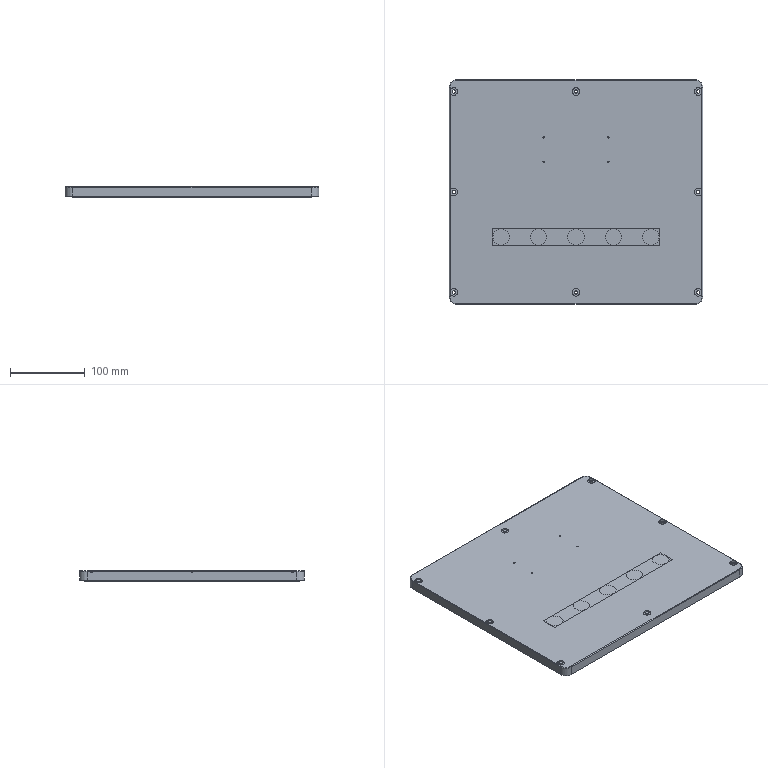Part | 2 solids | 125 faces | box 338 x 300 x 14.5 mm | volume 656011 mm3 | cylinder 57 | plane 52 | cone 12 | torus 4 | commonest cylinder face diameters 10 x10 4.5 x8 20 x8 6 x6 22 x5 2 x4